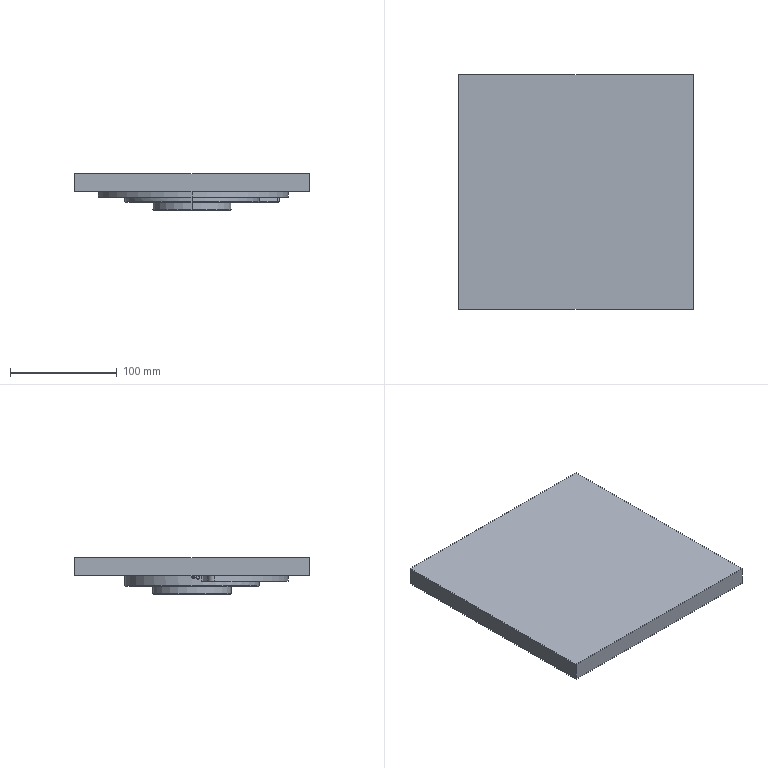NC program | NX | posted with a generic post | part box 220 x 220 x 34.5 mm
Whole program:
N10 G17 G21 G94 G90
(ADAPTIVE_MILLING_COPY , TOOL : D10)
N12 T03 M6
N14 G54
N16 G17 G0 G90 X2.716 Y17.888 S8000 M3
N18 G43 Z30. H3
N20 Z3.
N22 G94 G3 X2.716 Y17.888 Z2.506 I4.346 J1.167 F1000.
N24 X2.716 Y17.888 Z2.013 I4.346 J1.167
N26 X2.716 Y17.888 Z1.519 I4.346 J1.167
N28 X2.716 Y17.888 Z1.026 I4.346 J1.167
N30 X2.716 Y17.888 Z0.532 I4.346 J1.167
N32 X2.716 Y17.888 Z0.039 I4.346 J1.167
N34 X2.716 Y17.888 Z-0.455 I4.346 J1.167
N36 X2.716 Y17.888 Z-0.948 I4.346 J1.167
N38 X2.716 Y17.888 Z-1.442 I4.346 J1.167
N40 X2.716 Y17.888 Z-1.935 I4.346 J1.167
N42 X2.716 Y17.888 Z-2.429 I4.346 J1.167
N44 X2.716 Y17.888 Z-2.922 I4.346 J1.167
N46 X2.716 Y17.888 Z-3.416 I4.346 J1.167
N48 X2.716 Y17.888 Z-3.909 I4.346 J1.167
N50 X2.716 Y17.888 Z-4.403 I4.346 J1.167
N52 X2.716 Y17.888 Z-4.896 I4.346 J1.167
N54 X2.716 Y17.888 Z-5.39 I4.346 J1.167
N56 X2.716 Y17.888 Z-5.884 I4.346 J1.167
N58 X2.716 Y17.888 Z-6.377 I4.346 J1.167
N60 X2.562 Y19.055 Z-6.85 R-4.5
N62 X3.383 Y21.661 R-4.501 F3500.
N64 X8.053 Y14.188 R4.667
N66 X3.478 Y22.528 R-4.976
N68 X8.711 Y13.847 R5.194
N70 X3.384 Y23.139 R-5.476
N72 X9.145 Y13.448 R5.718
N74 X3.268 Y23.733 R-5.999
N76 X9.662 Y13.077 R6.259
N78 X3.411 Y24.511 R-6.54
N80 X10.277 Y12.751 R6.816
N82 X3.54 Y25.251 R-7.101
N84 X10.308 Y12.118 R7.391
N86 X3.277 Y25.774 R-7.685
N88 X9.662 Y11.224 R7.976
N90 X3.634 Y26.625 R-8.28
N92 X9.857 Y10.649 R8.582
N94 X3.931 Y27.41 R-8.89
N96 X9.362 Y9.854 R9.201
N98 X4.542 Y28.271 R-9.52
N100 X8.982 Y9.114 R9.839
N102 X5.936 Y29.188 R10.16
N104 X8.763 Y8.414 R-10.486
N106 X6.773 Y29.902 R10.813
N108 X6.843 Y7.627 R11.141
N110 X9.329 Y30.345 R11.47
N112 X4.111 Y7.333 R11.803
N114 X13.435 Y29.453 R12.135
N116 X-2.975 Y11.336 R12.452
N118 X19.934 Y19.603 R12.744
N120 X-3.247 Y27.048 R12.999
N122 X13.33 Y7.035 R13.282
N124 X3.629 Y32.267 R13.605
N126 X6.415 Y4.841 R13.939
N128 X10.361 Y33.004 R14.279
N130 X0.145 Y5.873 R14.618
N132 X20.504 Y25.811 R14.941
N134 X-7.945 Y22.137 R15.228
N136 X18.812 Y8.559 R15.508
N138 X0.809 Y33.635 R15.819
N140 X8.349 Y2.654 R16.156
N142 X8.223 Y35.578 R16.507
N144 X-0.93 Y3.92 R16.852
N146 X23.417 Y24.631 R17.169
N148 X-9.691 Y24.251 R17.446
N150 X19.666 Y6.189 R17.75
N152 X1.187 Y36.206 R18.081
N154 X6.266 Y0.364 R18.419
N156 X15.685 Y35.789 R18.757
N158 X-9.987 Y10.076 R19.08
N160 X26.272 Y15.384 R19.369
N162 X-1.406 Y36.84 R19.661
N164 X8.189 Y-1.19 R19.988
N166 X14.801 Y37.916 R20.325
N168 X-11.477 Y9.57 R20.641
N170 X27.88 Y15.462 R20.932
N172 X-5.392 Y36.339 R21.244
N174 X11.239 Y-2.415 R21.589
N176 X10.804 Y40.72 R21.927
N178 X-12.156 Y7.506 R22.236
N180 X29.663 Y16.717 R22.529
N182 X-12.155 Y31.619 R22.858
N184 X22.624 Y1.436 R23.224
N186 X0.916 Y41.898 R23.596
N188 X1.166 Y-4.412 R23.935
N190 X30.963 Y23.684 R24.215
N192 X-17.329 Y22.681 R24.515
N194 X29.606 Y7.931 R24.881
N196 X-7.054 Y40.094 R25.257
N198 X9.779 Y-6.692 R25.619
N200 X19.138 Y42.091 R25.939
N202 X-19.073 Y15.618 R26.215
N204 X32.436 Y10.504 R26.54
N206 X-9.113 Y40.665 R26.905
N208 X9.872 Y-8.332 R27.27
N210 X31.353 Y32.222 R27.545
N212 X-20.818 Y16.477 R27.828
N214 X34.139 Y10.383 R28.192
N216 X-13.922 Y38.615 R28.575
N218 X20.169 Y-7.081 R28.964
N220 X11.216 Y48.139 R29.325
N222 X-20.081 Y6.899 R29.589
N224 X37.112 Y17.241 R29.893
N226 X-20.334 Y32.265 R30.27
N228 X35.542 Y6.975 R-30.677
N230 X-10.353 Y44.912 R31.075
N232 X4.684 Y-12.514 R31.429
N234 X38.806 Y20.982 R31.66
N236 X-25.116 Y19.166 R31.992
N238 X38.939 Y12.068 R32.396
N240 X-19.377 Y38.683 R32.793
N242 X26.997 Y-7.815 R33.193
N244 X13.155 Y52.106 R33.559
N246 X-21.757 Y1.048 R33.807
N248 X41.256 Y15.873 R34.126
N250 X-27.369 Y23.479 R34.529
N252 X41.484 Y11.745 R34.949
N254 X-25.661 Y32.893 R35.364
N256 X40.899 Y6.65 R-35.786
N258 X-17.952 Y45.4 R36.198
N260 X8.094 Y-17.705 R36.567
N262 X38.936 Y37.722 R36.804
N264 X-30.067 Y15.176 R37.141
N266 X44.247 Y12.396 R37.546
N268 X13.492 Y56.405 R37.965
N270 X-30.525 Y25.606 R37.965
N272 X44.43 Y9.24 R38.393
N274 X-30.086 Y30.941 R38.821
N276 X44.886 Y7.691 R-39.249
N278 X-28.896 Y36.233 R39.678
N280 X25.894 Y-16.587 R40.091
N282 X22.285 Y56.567 R40.413
N284 X-28.702 Y-0.723 R40.677
N286 X47.754 Y25.827 R41.046
N288 X-34.57 Y20.407 R41.457
N290 X49.119 Y16.929 R41.882
N292 X-34.672 Y27.107 R42.31
N294 X48.583 Y7.952 R42.74
N296 X-32.704 Y36.316 R43.17
N298 X43.357 Y-5.524 R43.591
N300 X-14.118 Y57.762 R43.992
N302 X-10.658 Y-21.75 R44.316
N304 X49.466 Y33.391 R44.581
N306 X-38.078 Y20.459 R44.966
N308 X52.165 Y12.201 R45.389
N310 X-36.223 Y34.618 R45.814
N312 X44.975 Y-7.814 R46.231
N314 X-12.154 Y61.68 R46.627
N316 X-10.656 Y-24.618 R46.947
N318 X52.276 Y33.318 R47.227
N320 X-40.455 Y24.277 R47.612
N322 X54.035 Y7.978 R48.029
N324 X-35.913 Y41.814 R48.452
N326 X7.42 Y-29.926 R48.83
N328 X51.259 Y40.653 R49.041
N330 X-42.314 Y23.549 R49.391
N332 X56.226 Y9.748 R49.806
N334 X-39.088 Y39.358 R50.234
N336 X16.256 Y-30.894 R50.621
N338 X49.884 Y46.721 R50.846
N340 X-44.302 Y19.961 R51.179
N342 X58.321 Y11.441 R51.594
N344 X-41.303 Y38.717 R52.021
N346 X23.088 Y-31.032 R52.413
N348 X52.024 Y46.669 R52.636
N350 X-45.98 Y22.469 R52.961
N352 X54.68 Y-5.516 R53.364
N354 X-35.988 Y51.575 R53.772
N356 X16.02 Y-34.544 R54.152
N358 X56.534 Y42.013 R54.389
N360 X-47.429 Y25.976 R54.737
N362 X41.2 Y-24.486 R55.137
N364 X18.984 Y73.33 R55.465
N366 X-35.269 Y-17.545 R55.766
N368 X61.342 Y34.065 R56.129
N370 X-46.879 Y36.509 R56.511
N372 X29.501 Y-33.423 R56.893
N374 X55.176 Y50.08 R57.13
N376 X-50.244 Y25.13 R57.44
N378 X42.107 Y-27.178 R57.83
N380 X34.431 Y70.449 R58.131
N382 X-46.471 Y-4.811 R58.421
N384 X65.365 Y28.111 R58.801
N386 X-46.387 Y44.91 R59.193
N388 X32.199 Y-35.172 R59.575
N390 X57.762 Y51.058 R59.83
N392 X-53.222 Y21.694 R60.152
N394 X47.578 Y-26.178 R60.54
N396 X10.366 Y79.968 R60.874
N398 X-32.528 Y-27.865 R61.198
N400 X64.036 Y42.837 R61.557
N402 X-52.867 Y35.384 R61.929
N404 X45.069 Y-30.577 R62.315
N406 X44.879 Y69.094 R62.617
N408 X-53.301 Y0.64 R62.918
N410 X70.426 Y23.429 R63.308
N412 X-48.907 Y49.863 R63.706
N414 X34.131 Y-39.257 R64.089
N416 X60.612 Y54.983 R64.36
N418 X33.989 Y77.744 R63.941
N420 G1 X28.698 Y79.849
N422 X28.662 Y79.862
N424 G3 X20.997 Y82.139 R87.113
N426 X-54.045 Y-2.961 R64.765
N428 X48.665 Y-31.222 R65.099
N430 G2 X50.178 Y-29.197 R28.042
N432 X52.808 Y-27.177 R60.231
N434 G3 X60.417 Y-18.593 R46.468
N436 X49.891 Y68.594 R65.492
N438 G1 X48.977 Y69.287
N440 X48.946 Y69.309
N442 X44.187 Y72.436
N444 X44.154 Y72.455
N446 X39.195 Y75.254
N448 X39.161 Y75.272
N450 X36.229 Y76.674
N452 X24.021 Y81.354
N454 X23.204 Y81.615
N456 X17.64 Y82.995
N458 X11.996 Y83.997
N460 X7.521 Y84.475
N462 G3 X0.655 Y84.334 R43.981
N464 X-32.092 Y71.796 R65.284
N466 X-58.559 Y13.61 R65.788
N468 G1 X-58.529 Y13.481
N470 X-58.484 Y13.356
N472 X-58.099 Y12.813
N474 X-57.485 Y11.369
N476 X-57.205 Y9.883
N478 G3 X-57.255 Y6.281 R33.698
N480 X-55.034 Y-2.933 R40.231
N482 X46.954 Y-33.747 R66.001
N484 G1 X48.707 Y-31.16
N486 G3 X48.568 Y-30.401 R0.553
N488 G1 X48.189 Y-30.236 Z-6.829
N490 X47.8 Y-30.098 Z-6.809
N492 X46.7 Y-29.691 Z-6.75
N494 X-54.773 Y7.834
N496 X-56.597 Y8.505 Z-6.847
N498 X-56.652 Y8.516 Z-6.85
N500 G3 X-57.28 Y8.029 R0.552
N502 X-57.562 Y4.17 R25.827
N504 X-55.886 Y-3.248 R30.359
N506 X14.094 Y-47.609 R66.775
N508 X44.952 Y-36.336 R66.922
N510 X47.023 Y-33.645 R32.697
N512 X46.884 Y-32.886 R0.553
N514 G1 X46.507 Y-32.72 Z-6.829
N516 X46.119 Y-32.581 Z-6.809
N518 X45.018 Y-32.17 Z-6.75
N520 X-55.047 Y5.216
N522 X-56.868 Y5.894 Z-6.847
N524 X-56.923 Y5.905 Z-6.85
N526 G3 X-57.553 Y5.419 R0.552
N528 X-56.844 Y-3.055 R18.105
N530 X-47.8 Y-20.796 R61.927
N532 X42.848 Y-38.819 R67.936
N534 X44.964 Y-36.321 R29.568
N536 X44.849 Y-35.524 R0.552
N538 G1 X44.426 Y-35.342 Z-6.827
N540 X43.993 Y-35.186 Z-6.804
N542 X42.983 Y-34.808 Z-6.75
N544 X-55.263 Y1.938
N546 X-57.083 Y2.615 Z-6.847
N548 X-57.14 Y2.627 Z-6.85
N550 G3 X-57.77 Y2.096 R0.552
N552 X-57.77 Y-1.826 R30.463
N554 X-55.602 Y-8.983 R28.364
N556 X-16.913 Y-45.467 R68.138
N558 X40.552 Y-41.236 R68.868
N560 G1 X42.876 Y-38.789
N562 G3 X42.784 Y-37.954 R0.552
N564 G1 X42.272 Y-37.738 Z-6.822
N566 X41.75 Y-37.547 Z-6.794
N568 X40.92 Y-37.233 Z-6.75
N570 X-55.33 Y-0.82
N572 X-57.149 Y-0.135 Z-6.847
N574 X-57.204 Y-0.123 Z-6.85
N576 G3 X-57.84 Y-0.653 R0.552
N578 G1 X-57.844 Y-0.817
N580 X-57.843 Y-0.847
N582 X-57.817 Y-1.329
N584 G3 X-57.502 Y-5.564 R38.929
N586 X-54.651 Y-13.147 R30.654
N588 X-0.182 Y-50.379 R69.435
N590 X37.85 Y-43.693 R69.779
N592 X40.625 Y-41.159 R57.486
N594 X40.529 Y-40.321 R0.552
N596 G1 X40.016 Y-40.108 Z-6.822
N598 X39.493 Y-39.919 Z-6.794
N600 X38.661 Y-39.608 Z-6.75
N602 X-55.129 Y-4.569
N604 X-56.064 Y-4.215 Z-6.8
N606 X-57.005 Y-3.878 Z-6.85
N608 G3 X-57.649 Y-4.449 R0.552
N610 X-56.899 Y-9.724 R29.781
N612 X-53.157 Y-17.747 R36.163
N614 X34.904 Y-46.072 R70.603
N616 X37.854 Y-43.69 R29.715
N618 X37.766 Y-42.805 R0.551
N620 G1 X35.894 Y-42.101 Z-6.75
N622 X-54.654 Y-8.467
N624 X-56.53 Y-7.775 Z-6.85
N626 G3 X-57.198 Y-8.383 R0.551
N628 X-55.894 Y-14.167 R25.106
N630 X-50.72 Y-23.133 R44.051
N632 X31.686 Y-48.351 R71.626
N634 X34.937 Y-46.048 R32.018
N636 X34.839 Y-45.111 R0.551
N638 G1 X32.962 Y-44.42 Z-6.75
N640 X-53.857 Y-12.553
N642 X-55.735 Y-11.865 Z-6.85
N644 G3 X-56.437 Y-12.505 R0.551
N646 X-54.12 Y-19.416 R23.57
N648 X-45.519 Y-30.887 R56.893
N650 X28.12 Y-50.522 R72.643
N652 X31.778 Y-48.293 R44.276
N654 X31.649 Y-47.303 R0.551
N656 G1 X29.77 Y-46.619 Z-6.75
N658 X-52.751 Y-16.584
N660 X-54.631 Y-15.9 Z-6.85
N662 G3 X-55.382 Y-16.561 R0.552
N664 X-52.775 Y-23.11 R26.971
N666 X-44.509 Y-33.264 R54.486
N668 X24.096 Y-52.568 R73.579
N670 X28.148 Y-50.507 R58.714
N672 X28.079 Y-49.502 R0.551
N674 G1 X27.96 Y-49.459
N676 X26.078 Y-48.782 Z-6.75
N678 X-51.16 Y-21.
N680 X-53.042 Y-20.323 Z-6.85
N682 G3 X-53.84 Y-20.561 R0.584
N684 X-53.857 Y-20.997 R0.574
N686 X-50.497 Y-27.756 R29.648
N688 X-40.677 Y-38.034 R58.333
N690 X19.4 Y-54.467 R74.543
N692 G1 X20.294 Y-54.173
N694 X20.337 Y-54.156
N696 X24.137 Y-52.55
N698 G3 X24.107 Y-51.526 R0.551
N700 G1 X23.854 Y-51.436
N702 X21.969 Y-50.766 Z-6.75
N704 X-49.082 Y-25.512
N706 X-50.966 Y-24.843 Z-6.85
N708 X-51.199 Y-24.761
N710 X-51.445 Y-24.737
N712 G3 X-51.869 Y-25.52 R0.551
N714 X-48.329 Y-31.628 R40.408
N716 X-40.346 Y-39.52 R50.034
N718 X13.863 Y-56.115 R75.438
N720 G1 X15.777 Y-55.656
N722 X15.822 Y-55.643
N724 X19.503 Y-54.433
N726 G3 X19.513 Y-53.391 R0.55
N728 G1 X19.067 Y-53.235
N730 X17.18 Y-52.573 Z-6.75
N732 X-46.272 Y-30.31
N734 X-48.159 Y-29.647 Z-6.85
N736 X-48.681 Y-29.472
N738 G3 X-49.252 Y-30.291 R0.551
N740 G1 X-48.798 Y-31.068
N742 X-48.775 Y-31.106
N744 X-46.194 Y-34.823
N746 X-46.167 Y-34.858
N748 G3 X-39.576 Y-41.312 R36.113
N750 X7.33 Y-57.354 R76.215
N752 G1 X11.154 Y-56.764
N754 X11.2 Y-56.755
N756 X13.874 Y-56.113
N758 G3 X13.92 Y-55.057 R0.55
N760 G1 X13.176 Y-54.807
N762 X11.28 Y-54.171 Z-6.75
N764 X-41.641 Y-36.428
N766 X-43.538 Y-35.792 Z-6.85
N768 X-44.386 Y-35.515
N770 G3 X-44.901 Y-36.406 R0.551
N772 G1 X-43.302 Y-38.36
N774 X-43.272 Y-38.393
N776 X-40.139 Y-41.658
N778 X-40.107 Y-41.689
N780 G3 X-31.074 Y-48.139 R47.059
N782 X-1.616 Y-57.787 R77.307
N784 G1 X1.714 Y-57.824
N786 X1.76 Y-57.822
N788 X6.456 Y-57.488
N790 X6.502 Y-57.483
N792 X7.367 Y-57.349
N794 G3 X7.446 Y-56.28 R0.55
N796 G1 X5.785 Y-55.764
N798 X3.875 Y-55.171 Z-6.75
N800 X-34.475 Y-43.257
N802 X-36.385 Y-42.664 Z-6.85
N804 X-38.076 Y-42.146
N806 G3 X-38.519 Y-43.101 R0.55
N808 G1 X-36.726 Y-44.696
N810 X-36.691 Y-44.724
N812 X-33.083 Y-47.455
N814 X-33.047 Y-47.481
N816 X-29.235 Y-49.919
N818 X-29.196 Y-49.941
N820 X-25.203 Y-52.07
N822 X-25.163 Y-52.09
N824 X-21.015 Y-53.897
N826 X-20.974 Y-53.913
N828 X-16.695 Y-55.388
N830 X-16.653 Y-55.4
N832 X-12.272 Y-56.533
N834 X-12.228 Y-56.542
N836 X-7.772 Y-57.325
N838 X-7.727 Y-57.331
N840 X-3.039 Y-57.769
N842 X-2.993 Y-57.772
N844 X-1.493 Y-57.788
N846 X-1.352 Y-57.768
N848 X-1.218 Y-57.718
N850 X1.509 Y-56.188
N852 X3.254 Y-55.21 Z-6.75
N854 X45.409 Y-31.565
N856 X47.154 Y-30.587 Z-6.85
N858 X51.374 Y-28.22
N860 X51.396 Y-28.208
N862 G3 X54.205 Y-26.698 R21.883
N864 X59.618 Y-21.184 R28.83
N866 X72.222 Y31.316 R65.863
N868 X57.005 Y62.807 R66.863
N870 X49.829 Y68.64 R80.223
N872 X48.949 Y68.134 R0.552
N874 G1 X49.016 Y66.135 Z-6.75
N876 X52.054 Y-25.113
N878 X52.122 Y-27.053 Z-6.847
N880 X52.133 Y-27.111 Z-6.85
N882 G3 X52.8 Y-27.508 R0.553
N884 X56.743 Y-25.459 R8.272
N886 X62.894 Y-18.253 R36.756
N888 X61.924 Y58.007 R67.156
N890 G1 X61.898 Y58.034
N892 X57.866 Y62.056
N894 X57.838 Y62.082
N896 X56.99 Y62.82
N898 G3 X56.077 Y62.375 R0.553
N900 G1 X56.008 Y60.376 Z-6.75
N902 X53.031 Y-24.859
N904 X52.966 Y-26.8 Z-6.847
N906 X52.973 Y-26.858 Z-6.85
N908 G3 X53.649 Y-27.295 R0.552
N910 G1 X54.263 Y-27.141
N912 X54.324 Y-27.132
N914 X54.449 Y-27.129
N916 X54.573 Y-27.115
N918 X54.696 Y-27.093
N920 X54.818 Y-27.066
N922 X54.94 Y-27.037
N924 X55.06 Y-27.003
N926 X55.179 Y-26.965
N928 G3 X59.07 Y-24.303 R11.344
N930 X66.021 Y-15.028 R44.175
N932 X66.244 Y52.98 R68.174
N934 G1 X65.7 Y53.693
N936 X65.676 Y53.722
N938 X62.053 Y57.86
N940 G3 X61.091 Y57.545 R0.551
N942 G1 X61.077 Y57.386
N944 X60.907 Y55.394 Z-6.75
N946 X54.049 Y-24.636
N948 X53.886 Y-26.629 Z-6.85
N950 G3 X54.449 Y-27.129 R0.553
N952 X58.177 Y-25.911 R5.856
N954 X63.347 Y-20.693 R24.137
N956 X73.335 Y-0.385 R64.082
N958 X69.673 Y48.381 R69.131
N960 X66.197 Y53.041 R83.217
N962 X65.215 Y52.779 R0.551
N964 G1 X65.189 Y52.587
N966 X64.928 Y50.604 Z-6.75
N968 X55.012 Y-24.598
N970 X54.759 Y-26.581 Z-6.85
N972 G3 X55.323 Y-27.106 R0.553
N974 X59.038 Y-26.039 R5.782
N976 X64.205 Y-21.002 R21.991
N978 X72.844 Y-4.862 R61.211
N980 X72.539 Y43.992 R70.021
N982 X69.628 Y48.45 R396.035
N984 X68.627 Y48.242 R0.551
N986 G1 X68.586 Y48.01
N988 X68.239 Y46.041 Z-6.75
N990 X55.786 Y-24.574
N992 X55.445 Y-26.544 Z-6.85
N994 G3 X55.889 Y-27.097 R0.554
N996 X59.032 Y-26.658 R4.332
N998 X63.769 Y-22.834 R15.987
N1000 X70.769 Y-12.074 R48.624
N1002 X75.005 Y39.652 R70.807
N1004 G1 X72.535 Y44.
N1006 G3 X71.52 Y43.846 R0.551
N1008 G1 X71.459 Y43.568
N1010 X71.03 Y41.614 Z-6.75
N1012 X56.489 Y-24.651
N1014 X56.063 Y-26.605 Z-6.85
N1016 G3 X56.502 Y-27.217 R0.553
N1018 X60.01 Y-26.768 R4.73
N1020 X64.924 Y-22.769 R16.622
N1022 X71.749 Y-12.191 R47.773
N1024 X77.137 Y35.275 R71.619
N1026 G1 X75.147 Y39.399
N1028 X75.13 Y39.433
N1030 X74.944 Y39.759
N1032 G3 X73.934 Y39.625 R0.551
N1034 G1 X73.856 Y39.323
N1036 X73.356 Y37.387 Z-6.75
N1038 X57.296 Y-24.808
N1040 X56.799 Y-26.745 Z-6.85
N1042 G3 X57.238 Y-27.361 R0.553
N1044 X60.232 Y-27.227 R4.02
N1046 X65.173 Y-23.689 R14.26
N1048 X71.427 Y-14.831 R41.208
N1050 X78.939 Y30.994 R72.072
N1052 X77.116 Y35.318 R55.462
N1054 X76.095 Y35.239 R0.551
N1056 G1 X76.011 Y34.964
N1058 X75.43 Y33.051 Z-6.75
N1060 X57.813 Y-24.907
N1062 X57.232 Y-26.821 Z-6.85
N1064 G3 X57.545 Y-27.456 R0.554
N1066 X60.577 Y-27.622 R3.764
N1068 X65.396 Y-24.575 R12.82
N1070 X71.759 Y-16.114 R36.775
N1072 X80.785 Y22.207 R71.989
N1074 X80.445 Y26.838 R122.758
N1076 X78.938 Y30.994 R40.273
N1078 X77.908 Y30.969 R0.551
N1080 G1 X77.801 Y30.66
N1082 X77.147 Y28.77 Z-6.75
N1084 X58.476 Y-25.127
N1086 X57.821 Y-27.017 Z-6.85
N1088 G3 X58.118 Y-27.708 R0.553
N1090 X61.391 Y-27.882 R4.062
N1092 X66.411 Y-24.688 R13.321
N1094 X72.82 Y-16.105 R36.835
N1096 X81.79 Y19.38 R72.433
N1098 G1 X81.787 Y19.88
N1100 X81.781 Y20.38
N1102 X81.772 Y20.879
N1104 X81.76 Y21.379
N1106 X81.743 Y21.879
N1108 X81.728 Y22.254
N1110 X81.701 Y22.814
N1112 G3 X80.413 Y26.937 R62.817
N1114 X79.377 Y26.965 R0.551
N1116 G1 X79.234 Y26.594
N1118 X78.512 Y24.729 Z-6.75
N1120 X59.115 Y-25.404
N1122 X58.393 Y-27.269 Z-6.85
N1124 G3 X58.69 Y-27.959 R0.553
N1126 X61.76 Y-28.286 R3.815
N1128 X66.709 Y-25.463 R12.335
N1130 X72.944 Y-17.695 R32.876
N1132 X81.544 Y5.77 R70.004
N1134 X82.728 Y18.763 R77.216
N1136 G1 X81.684 Y22.882
N1138 G3 X80.646 Y22.966 R0.55
N1140 G1 X80.46 Y22.536
N1142 X79.666 Y20.7 Z-6.75
N1144 X59.633 Y-25.628
N1146 X58.84 Y-27.464 Z-6.85
N1148 G3 X59.07 Y-28.157 R0.554
N1150 X62.178 Y-28.683 R3.814
N1152 X67.219 Y-26.036 R11.879
N1154 X73.715 Y-18.165 R31.792
N1156 X82.041 Y3.425 R68.847
N1158 X83.539 Y14.599 R78.021
N1160 X82.714 Y18.818 R64.758
N1162 X81.685 Y18.92 R0.551
N1164 G1 X81.484 Y18.499
N1166 X80.622 Y16.694 Z-6.75
N1168 X60.256 Y-25.942
N1170 X59.394 Y-27.747 Z-6.85
N1172 G3 X59.611 Y-28.47 R0.554
N1174 X62.958 Y-29.019 R4.048
N1176 X68.102 Y-26.298 R12.318
N1178 X74.543 Y-18.542 R31.69
N1180 X82.655 Y1.807 R68.753
N1182 X84.143 Y10.6 R79.303
N1184 X83.52 Y14.703 R38.965
N1186 X82.491 Y14.859 R0.551
N1188 G1 X82.281 Y14.457
N1190 X81.356 Y12.684 Z-6.75
N1192 X60.968 Y-26.352
N1194 X60.042 Y-28.125 Z-6.85
N1196 G3 X60.261 Y-28.845 R0.553
N1198 X63.613 Y-29.392 R4.146
N1200 X68.983 Y-26.573 R12.602
N1202 X75.691 Y-18.395 R32.519
N1204 X83.555 Y1.523 R68.964
N1206 X84.574 Y6.833 R76.032
N1208 G1 X84.133 Y10.683
N1210 G3 X83.109 Y10.893 R0.55
N1212 G1 X82.846 Y10.433
N1214 X81.852 Y8.698 Z-6.75
N1216 X61.576 Y-26.703
N1218 X60.583 Y-28.439 Z-6.85
N1220 G3 X60.802 Y-29.157 R0.553
N1222 X64.386 Y-29.752 R4.321
N1224 X69.955 Y-26.779 R13.154
N1226 X76.766 Y-18.363 R33.391
N1228 X84.77 Y2.666 R70.068
N1230 G1 X84.577 Y6.786
N1232 G3 X83.578 Y7.047 R0.541
N1234 G1 X83.169 Y6.39
N1236 X82.112 Y4.693 Z-6.75
N1238 X62.297 Y-27.118
N1240 X61.241 Y-28.817 Z-6.85
N1242 G3 X61.451 Y-29.532 R0.543
N1244 X65.036 Y-30.145 R4.367
N1246 X70.538 Y-27.308 R13.1
N1248 X77.387 Y-19.086 R32.713
N1250 X84.793 Y-1.298 R68.093
N1252 X84.766 Y2.768 R39.621
N1254 X83.761 Y3.051 R0.55
N1256 G1 X83.288 Y2.354
N1258 X82.164 Y0.699 Z-6.75
N1260 X63.004 Y-27.527
N1262 X61.884 Y-29.184 Z-6.85
N1264 G3 X62.101 Y-29.907 R0.553
N1266 X65.683 Y-30.546 R4.421
N1268 X71.406 Y-27.603 R13.294
N1270 X78.131 Y-19.6 R32.453
N1272 X84.686 Y-5.036 R65.018
N1274 X84.796 Y-1.174 R181.103
N1276 X83.804 Y-0.835 R0.55
N1278 G1 X83.404 Y-1.375
N1280 X82.213 Y-2.982 Z-6.75
N1282 X63.722 Y-27.941
N1284 X62.538 Y-29.552 Z-6.85
N1286 G3 X62.751 Y-30.282 R0.553
N1288 X66.453 Y-30.926 R4.533
N1290 X72.085 Y-28.067 R13.517
N1292 X78.938 Y-20.011 R32.265
N1294 X84.35 Y-8.866 R61.683
N1296 G1 X84.689 Y-5.005
N1298 G3 X83.714 Y-4.611 R0.55
N1300 G1 X83.301 Y-5.119
N1302 X82.041 Y-6.673 Z-6.75
N1304 X64.446 Y-28.358
N1306 X63.193 Y-29.917 Z-6.85
N1308 G3 X63.4 Y-30.657 R0.553
N1310 X67.099 Y-31.336 R4.566
N1312 X72.758 Y-28.533 R13.506
N1314 X79.678 Y-20.534 R32.182
N1316 X83.868 Y-12.564 R58.873
N1318 X84.352 Y-8.851 R38.627
N1320 X83.392 Y-8.437 R0.55
N1322 G1 X83.017 Y-8.86
N1324 X81.689 Y-10.355 Z-6.75
N1326 X65.277 Y-28.839
N1328 X63.987 Y-30.296 Z-6.847
N1330 X63.958 Y-30.342 Z-6.85
N1332 G3 X64.158 Y-31.095 R0.553
N1334 X67.742 Y-31.751 R4.539
N1336 X73.526 Y-28.925 R13.481
N1338 X80.614 Y-20.745 R32.444
N1340 X83.359 Y-15.83 R58.223
N1342 G1 X83.878 Y-12.496
N1344 G3 X82.943 Y-12.026 R0.55
N1346 G1 X82.545 Y-12.43
N1348 X81.144 Y-13.857 Z-6.75
N1350 X66.011 Y-29.263
N1352 X64.652 Y-30.651 Z-6.847
N1354 X64.619 Y-30.698 Z-6.85
N1356 G3 X64.807 Y-31.47 R0.552
N1358 X68.507 Y-32.149 R4.599
N1360 X74.491 Y-29.171 R13.926
N1362 X81.612 Y-20.853 R33.251
N1364 G1 X81.81 Y-20.535
N1366 X82.006 Y-20.215
N1368 X82.199 Y-19.894
N1370 X82.453 Y-19.463
N1372 X82.578 Y-19.246
N1374 X82.604 Y-19.191
N1376 X83.349 Y-15.884
N1378 X83.356 Y-15.847
N1380 X83.376 Y-15.723
N1382 G3 X82.458 Y-15.236 R0.551
N1384 G1 X82.003 Y-15.658
N1386 X80.538 Y-17.02 Z-6.75
N1388 X66.846 Y-29.746
N1390 X65.425 Y-31.07 Z-6.847
N1392 X65.389 Y-31.116 Z-6.85
N1394 G3 X65.565 Y-31.907 R0.552
N1396 X69.151 Y-32.568 R4.589
N1398 X75.062 Y-29.724 R13.636
N1400 X81.927 Y-22.009 R31.534
N1402 X82.628 Y-19.085 R62.911
N1404 X81.742 Y-18.539 R0.551
N1406 G1 X81.388 Y-18.831
N1408 X79.844 Y-20.102 Z-6.75
N1410 X67.599 Y-30.181
N1412 X66.099 Y-31.419 Z-6.847
N1414 X66.062 Y-31.46 Z-6.85
N1416 G3 X66.215 Y-32.282 R0.552
N1418 X69.917 Y-32.973 R4.683
N1420 X75.929 Y-30.054 R13.949
N1422 X81.146 Y-24.638 R28.596
N1424 G1 X81.929 Y-22.002
N1426 G3 X81.079 Y-21.4 R0.55
N1428 G1 X80.697 Y-21.677
N1430 X79.077 Y-22.851 Z-6.75
N1432 X68.357 Y-30.619
N1434 X66.743 Y-31.799 Z-6.85
N1436 G3 X66.864 Y-32.657 R0.552
N1438 X70.681 Y-33.38 R4.777
N1440 X76.698 Y-30.465 R14.136
N1442 X80.507 Y-26.788 R24.792
N1444 G1 X81.148 Y-24.631
N1446 G3 X80.324 Y-24.011 R0.551
N1448 G1 X80.043 Y-24.191
N1450 X78.358 Y-25.27 Z-6.75
N1452 X69.22 Y-31.118
N1454 X67.539 Y-32.201 Z-6.85
N1456 G3 X67.622 Y-33.095 R0.551
N1458 X71.321 Y-33.813 R4.718
N1460 X76.961 Y-31.251 R13.704
N1462 X79.754 Y-28.832 R18.88
N1464 G1 X80.474 Y-26.896
N1466 X80.486 Y-26.861
N1468 X80.521 Y-26.741
N1470 G3 X79.721 Y-26.106 R0.551
N1472 G1 X79.417 Y-26.28
N1474 X77.68 Y-27.272 Z-6.75
N1476 X70.08 Y-31.609
N1478 X68.344 Y-32.602 Z-6.85
N1480 G3 X68.38 Y-33.532 R0.551
N1482 X72.084 Y-34.225 R4.746
N1484 X77.829 Y-31.594 R13.989
N1486 X79.14 Y-30.485 R6.86
N1488 G1 X79.793 Y-28.727
N1490 G3 X79.035 Y-28.042 R0.551
N1492 G1 X78.823 Y-28.146
N1494 X77.028 Y-29.027 Z-6.75
N1496 X70.855 Y-32.057
N1498 X69.06 Y-32.938 Z-6.85
N1500 G3 X69.029 Y-33.907 R0.551
N1502 X72.847 Y-34.642 R4.847
N1504 X78.558 Y-31.963 R12.994
N1506 X79.153 Y-30.449 R20.278
N1508 X78.424 Y-29.75 R0.551
N1510 G1 X78.292 Y-29.806
N1512 X76.449 Y-30.582 Z-6.75
N1514 X71.735 Y-32.567
N1516 X69.892 Y-33.343 Z-6.85
N1518 G3 X69.787 Y-34.345 R0.552
N1520 X73.607 Y-35.061 R4.837
N1522 X77.968 Y-33.274 R11.136
N1524 X78.633 Y-31.847 R5.407
N1526 X77.93 Y-31.138 R0.551
N1528 G1 X70.551 Y-33.826
N1530 G3 X70.545 Y-34.782 R0.551
N1532 X74.122 Y-35.519 R4.708
N1534 X77.506 Y-34.31 R8.108
N1536 X78.122 Y-33.047 R6.467
N1538 X77.454 Y-32.297 R0.551
N1540 G1 X71.327 Y-34.254
N1542 G3 X71.303 Y-35.22 R0.551
N1544 X75.131 Y-35.898 R4.858
N1546 X77.112 Y-35.176 R5.182
N1548 X77.633 Y-34.134 R4.548
N1550 X76.999 Y-33.375 R0.551
N1552 G1 X72.013 Y-34.612
N1554 G3 X71.952 Y-35.595 R0.551
N1556 X76.797 Y-35.874 R4.503
N1558 X77.268 Y-34.944 R3.882
N1560 X76.648 Y-34.182 R0.551
N1562 G1 X72.782 Y-35.045
N1564 G3 X72.71 Y-36.032 R0.551
N1566 X76.377 Y-36.541 R3.866
N1568 G1 X76.662 Y-36.291
N1570 X76.918 Y-35.721
N1572 G3 X76.316 Y-34.954 R0.551
N1574 G1 X73.556 Y-35.476
N1576 G3 X73.468 Y-36.47 R0.551
N1578 X75.94 Y-37.054 R3.135
N1580 X76.673 Y-36.265 R1.04
N1582 X76.072 Y-35.498 R0.551
N1584 G1 X74.206 Y-35.851
N1586 G3 X74.117 Y-36.845 R0.551
N1588 X75.871 Y-37.327 R2.334
N1590 X76.484 Y-36.685 R0.859
N1592 X75.869 Y-35.921 R0.551
N1594 G1 X74.735 Y-36.168
N1596 G3 X74.658 Y-37.157 R0.551
N1598 X75.942 Y-37.482 R1.536
N1600 X76.342 Y-37.001 R0.823
N1602 X75.669 Y-36.252 R0.551
N1604 G1 X75.111 Y-36.444
N1606 G3 X75.091 Y-37.407 R0.551
N1608 X76.147 Y-37.4 R0.754
N1610 G1 X76.211 Y-37.293
N1612 X76.262 Y-37.179
N1614 G3 X75.923 Y-36.336 R0.642
N1616 X75.078 Y-36.679 R0.642
N1618 X75.359 Y-37.562 R0.691
N1620 X75.979 Y-37.544 R0.634
N1622 X76.182 Y-36.8 R0.553
N1624 G1 X75.778 Y-36.082
N1626 X74.798 Y-34.338 Z-6.75
N1628 X9.562 Y81.738
N1630 X8.582 Y83.482 Z-6.85
N1632 X8.142 Y84.251
N1634 G3 X7.77 Y84.456 R0.576
N1636 G1 X6.334 Y84.613
N1638 X6.296 Y84.615
N1640 X0.583 Y84.848
N1642 G3 X-10.154 Y83.348 R40.247
N1644 X-59.57 Y15.083 R66.563
N1646 X-59.013 Y14.088 R1.206
N1648 G1 X-58.427 Y13.278
N1650 G3 X-57.651 Y13.161 R0.553
N1652 G1 X-57.377 Y13.469 Z-6.829
N1654 X-57.125 Y13.795 Z-6.809
N1656 X-56.394 Y14.715 Z-6.75
N1658 X-2.772 Y82.249
N1660 X-1.528 Y83.816 Z-6.85
N1662 G3 X-1.916 Y84.781 R0.558
N1664 X-10.62 Y84.041 R48.968
N1666 X-25.036 Y78.475 R57.326
N1668 X-60.584 Y16.78 R67.519
N1670 X-60.254 Y15.204 R3.73
N1672 G1 X-60.216 Y15.156
N1674 X-60.184 Y15.133
N1676 X-59.341 Y14.388
N1678 G3 X-58.602 Y14.397 R0.554
N1680 G1 X-58. Y15.196 Z-6.8
N1682 X-57.417 Y16.007 Z-6.75
N1684 X-9.528 Y81.758
N1686 X-8.35 Y83.375 Z-6.85
N1688 G3 X-8.292 Y84.149 R0.595
N1690 X-8.771 Y84.35 R0.561
N1692 X-16.519 Y83.099 R48.801
N1694 X-28.734 Y77.436 R53.541
N1696 X-61.551 Y18.288 R68.457
N1698 X-61.075 Y15.725 R6.667
N1700 X-60.184 Y15.133 R2.829
N1702 X-59.486 Y15.186 R0.554
N1704 G1 X-59.107 Y15.717 Z-6.817
N1706 X-58.748 Y16.264 Z-6.785
N1708 X-58.363 Y16.839 Z-6.75
N1710 X-15.477 Y80.856
N1712 X-14.364 Y82.518 Z-6.85
N1714 G3 X-14.18 Y83.003 R0.735
N1716 X-14.817 Y83.505 R0.552
N1718 X-21.855 Y81.875 R49.543
N1720 X-31.969 Y76.458 R48.761
N1722 X-62.485 Y19.723 R69.341
N1724 X-61.944 Y16.289 R8.96
N1726 X-61.554 Y15.898 R0.785
N1728 G1 X-60.898 Y15.535
N1730 G3 X-60.181 Y15.702 R0.554
N1732 G1 X-59.136 Y17.408 Z-6.75
N1734 X-21.1 Y79.581
N1736 X-20.056 Y81.287 Z-6.85
N1738 X-19.938 Y81.486
N1740 X-19.87 Y81.706
N1742 G3 X-20.543 Y82.286 R0.551
N1744 X-26.974 Y80.319 R43.935
N1746 X-36.08 Y74.649 R47.615
N1748 X-63.394 Y21.091 R70.287
N1750 X-62.855 Y16.901 R11.531
N1752 X-62.273 Y16.115 R1.432
N1754 G1 X-61.611 Y15.922
N1756 G3 X-60.996 Y16.149 R0.555
N1758 G1 X-60.014 Y17.891 Z-6.75
N1760 X-26.16 Y78.058
N1762 X-25.179 Y79.801 Z-6.85
N1764 G3 X-24.983 Y80.274 R1.1
N1766 X-25.694 Y80.82 R0.551
N1768 X-32.082 Y78.359 R35.485
N1770 X-41.832 Y70.989 R51.684
N1772 X-64.283 Y22.272 R71.086
N1774 X-63.797 Y17.57 R14.192
N1776 X-63.121 Y16.391 R2.851
N1778 G1 X-63.016 Y16.332
N1780 X-62.176 Y16.087
N1782 G3 X-61.506 Y16.415 R0.559
N1784 G1 X-60.593 Y18.194 Z-6.75
N1786 X-30.762 Y76.346
N1788 X-29.849 Y78.126 Z-6.85
N1790 X-29.736 Y78.342
N1792 X-29.652 Y78.571
N1794 G3 X-30.392 Y79.168 R0.551
N1796 X-36.189 Y76.582 R34.927
N1798 X-44.359 Y69.825 R47.
N1800 X-65.154 Y23.521 R71.888
N1802 X-64.687 Y18.068 R16.41
N1804 X-63.851 Y16.552 R3.669
N1806 X-62.953 Y16.314 R3.201
N1808 X-62.279 Y16.654 R0.557
N1810 G1 X-61.431 Y18.466 Z-6.75
N1812 X-35.268 Y74.361
N1814 X-34.42 Y76.173 Z-6.85
N1816 X-34.298 Y76.424
N1818 X-34.211 Y76.689
N1820 G3 X-34.988 Y77.25 R0.551
N1822 X-39.671 Y74.926 R41.794
N1824 X-46.69 Y68.743 R40.451
N1826 X-66.015 Y24.591 R72.644
N1828 X-65.606 Y18.632 R18.423
N1830 X-64.564 Y16.671 R4.204
N1832 X-63.654 Y16.453 R2.912
N1834 X-63.018 Y16.861 R0.57
N1836 G1 X-62.232 Y18.7 Z-6.75
N1838 X-39.334 Y72.289
N1840 X-38.548 Y74.128 Z-6.85
N1842 X-38.339 Y74.637
N1844 G3 X-39.137 Y75.25 R0.551
N1846 X-43.481 Y72.78 R53.383
N1848 X-49.827 Y66.604 R38.362
N1850 X-66.896 Y25.212 R73.211
N1852 X-66.479 Y19.004 R19.415
N1854 X-65.339 Y16.813 R4.773
N1856 X-64.293 Y16.566 R3.199
N1858 X-63.651 Y16.995 R0.573
N1860 G1 X-62.917 Y18.856 Z-6.75
N1862 X-42.561 Y70.464
N1864 X-41.827 Y72.325 Z-6.85
N1866 X-41.627 Y72.854
N1868 G3 X-42.428 Y73.453 R0.551
N1870 X-47.343 Y70.277 R44.052
N1872 X-53.452 Y63.526 R39.968
N1874 X-67.739 Y26.296 R73.915
N1876 X-67.414 Y19.582 R21.58
N1878 X-66.192 Y17.013 R5.751
N1880 G1 X-66.095 Y16.935
N1882 X-65.985 Y16.876
N1884 X-65.936 Y16.856
N1886 X-65.074 Y16.704
N1888 G3 X-64.439 Y17.121 R0.56
N1890 G1 X-63.77 Y19.006 Z-6.75
N1892 X-46.356 Y68.046
N1894 X-45.687 Y69.931 Z-6.85
N1896 X-45.505 Y70.465
N1898 G3 X-46.342 Y71.025 R0.551
N1900 X-51.42 Y67.223 R28.176
N1902 X-58.073 Y58.336 R49.565
N1904 X-68.59 Y27.21 R74.595
N1906 X-68.312 Y19.995 R23.487
N1908 X-67.021 Y17.184 R6.416
N1910 G1 X-66.929 Y17.099
N1912 X-66.822 Y17.034
N1914 X-66.732 Y16.996
N1916 X-65.871 Y16.844
N1918 G3 X-65.24 Y17.252 R0.555
N1920 G1 X-64.635 Y19.159 Z-6.75
N1922 X-49.952 Y65.418
N1924 X-49.347 Y67.324 Z-6.85
N1926 X-49.156 Y67.95
N1928 G3 X-50.026 Y68.475 R0.551
N1930 X-53.844 Y65.48 R36.5
N1932 X-59.258 Y58.161 R38.368
N1934 X-69.447 Y27.953 R74.844
N1936 X-69.2 Y20.364 R24.544
N1938 X-67.826 Y17.32 R6.699
N1940 G1 X-67.733 Y17.237
N1942 X-67.625 Y17.173
N1944 X-67.545 Y17.139
N1946 X-66.683 Y16.987
N1948 G3 X-66.055 Y17.389 R0.554
N1950 G1 X-65.509 Y19.313 Z-6.75
N1952 X-53.145 Y62.835
N1954 X-52.599 Y64.759 Z-6.85
N1956 X-52.394 Y65.507
N1958 G3 X-53.295 Y65.991 R0.551
N1960 X-56.871 Y62.868 R53.342
N1962 X-61.516 Y56.072 R35.229
N1964 X-70.32 Y28.502 R74.701
N1966 X-70.08 Y20.663 R25.395
N1968 X-68.676 Y17.496 R7.148
N1970 G1 X-68.588 Y17.407
N1972 X-68.485 Y17.337
N1974 X-68.364 Y17.284
N1976 X-67.502 Y17.132
N1978 G3 X-66.876 Y17.529 R0.554
N1980 G1 X-66.382 Y19.467 Z-6.75
N1982 X-55.937 Y60.393
N1984 X-55.443 Y62.331 Z-6.85
N1986 X-55.254 Y63.097
N1988 G3 X-56.157 Y63.568 R0.551
N1990 X-60.231 Y59.546 R33.885
N1992 X-64.725 Y51.768 R42.165
N1994 X-71.262 Y28.276 R72.78
N1996 X-70.839 Y20.449 R23.715
N1998 X-69.425 Y17.561 R6.504
N2000 G1 X-69.323 Y17.489
N2002 X-69.194 Y17.43
N2004 X-68.332 Y17.278
N2006 G3 X-67.707 Y17.671 R0.554
N2008 G1 X-67.275 Y19.624 Z-6.75
N2010 X-58.91 Y57.509
N2012 X-58.479 Y59.462 Z-6.85
N2014 X-58.313 Y60.249
N2016 G3 X-59.245 Y60.675 R0.551
N2018 X-62.961 Y56.657 R28.966
N2020 X-67.369 Y47.982 R44.609
N2022 X-72.17 Y28.38 R70.625
N2024 X-71.68 Y20.558 R23.568
N2026 X-70.233 Y17.687 R6.369
N2028 X-69.161 Y17.424 R2.945
N2030 X-68.537 Y17.816 R0.554
N2032 G1 X-68.167 Y19.781 Z-6.75
N2034 X-61.693 Y54.473
N2036 X-61.326 Y56.439 Z-6.85
N2038 X-61.161 Y57.363
N2040 G3 X-62.119 Y57.744 R0.551
N2042 X-65.15 Y54.253 R46.518
N2044 X-68.825 Y46.75 R35.86
N2046 X-73.071 Y28.547 R68.238
N2048 X-72.539 Y20.728 R23.42
N2050 X-71.098 Y17.852 R6.579
N2052 X-70.009 Y17.574 R2.699
N2054 X-69.385 Y17.966 R0.554
N2056 G1 X-69.065 Y19.94 Z-6.75
N2058 X-63.974 Y51.783
N2060 X-63.658 Y53.758 Z-6.85
N2062 X-63.502 Y54.776
N2064 G3 X-64.461 Y55.143 R0.551
N2066 X-67.874 Y50.701 R39.423
N2068 X-71.245 Y42.511 R40.01
N2070 X-74.034 Y27.559 R60.246
N2072 X-73.208 Y20.27 R20.865
N2074 X-71.941 Y17.996 R5.976
N2076 X-70.857 Y17.723 R2.802
N2078 X-70.231 Y18.117 R0.554
N2080 G1 X-69.981 Y20.101 Z-6.75
N2082 X-66.484 Y48.578
N2084 X-66.24 Y50.563 Z-6.85
N2086 X-66.129 Y51.527
N2088 G3 X-67.111 Y51.844 R0.551
N2090 X-70.519 Y46.792 R26.535
N2092 X-73.789 Y36.444 R49.027
N2094 X-74.894 Y25.031 R43.706
N2096 X-73.558 Y19.224 R14.897
N2098 X-72.646 Y18.056 R2.94
N2100 G1 X-72.577 Y18.027
N2102 X-71.715 Y17.875
N2104 G3 X-71.088 Y18.274 R0.554
N2106 G1 X-70.915 Y20.266 Z-6.75
N2108 X-68.859 Y45.091
N2110 X-68.694 Y47.084 Z-6.85
N2112 X-68.612 Y48.169
N2114 G3 X-69.615 Y48.434 R0.551
N2116 X-72.075 Y44.669 R43.462
N2118 X-74.77 Y36.237 R36.268
N2120 X-75.751 Y24.816 R41.433
N2122 X-74.363 Y19.276 R14.406
N2124 X-73.515 Y18.213 R3.024
N2126 G1 X-73.429 Y18.177
N2128 X-72.567 Y18.025
N2130 G3 X-71.939 Y18.43 R0.553
N2132 G1 X-71.874 Y19.328 Z-6.805
N2134 X-71.833 Y20.227 Z-6.76
N2136 X-71.823 Y20.426 Z-6.75
N2138 X-70.676 Y42.171
N2140 X-70.57 Y44.168 Z-6.85
N2142 X-70.513 Y45.395
N2144 G3 X-71.514 Y45.644 R0.551
N2146 X-74.179 Y41.001 R50.135
N2148 X-76.5 Y31.181 R35.346
N2150 X-76.249 Y22.346 R28.571
N2152 X-74.727 Y18.682 R9.012
N2154 X-74.288 Y18.328 R1.502
N2156 G1 X-73.426 Y18.176
N2158 G3 X-72.795 Y18.594 R0.553
N2160 G1 X-72.771 Y19.198 Z-6.82
N2162 X-72.775 Y19.802 Z-6.79
N2164 X-72.77 Y20.592 Z-6.75
N2166 X-72.672 Y38.666
N2168 X-72.661 Y40.666 Z-6.85
N2170 X-72.662 Y41.816
N2172 G3 X-73.679 Y42.009 R0.551
N2174 X-76.213 Y36.89 R27.724
N2176 X-77.232 Y23.049 R30.796
N2178 X-75.707 Y18.984 R10.285
N2180 X-75.146 Y18.48 R1.51
N2182 G1 X-74.284 Y18.328
N2184 G3 X-73.649 Y18.765 R0.553
N2186 G1 X-73.653 Y19.274 Z-6.825
N2188 X-73.685 Y19.781 Z-6.799
N2190 X-73.736 Y20.762 Z-6.75
N2192 X-74.476 Y35.089
N2194 X-74.58 Y37.086 Z-6.85
N2196 X-74.642 Y38.158
N2198 G3 X-75.671 Y38.288 R0.551
N2200 X-77.499 Y34.349 R30.085
N2202 X-77.792 Y21.873 R24.111
N2204 X-76.249 Y18.77 R7.175
N2206 G1 X-76.148 Y18.696
N2208 X-76.035 Y18.642
N2210 X-76.012 Y18.632
N2212 X-75.027 Y18.459
N2214 G3 X-74.386 Y18.933 R0.552
N2216 G1 X-74.422 Y19.439 Z-6.825
N2218 X-74.486 Y19.943 Z-6.799
N2220 X-74.597 Y20.92 Z-6.75
N2222 X-75.855 Y31.931
N2224 X-76.082 Y33.919 Z-6.85
N2226 X-76.212 Y34.991
N2228 G3 X-77.246 Y35.056 R0.551
N2230 X-78.737 Y31.347 R35.908
N2232 X-78.228 Y20.762 R18.395
N2234 X-77.046 Y18.87 R5.188
N2236 X-75.892 Y18.611 R4.
N2238 X-75.248 Y19.115 R0.552
N2240 G1 X-75.317 Y19.666 Z-6.822
N2242 X-75.414 Y20.214 Z-6.794
N2244 X-75.557 Y21.089 Z-6.75
N2246 X-76.914 Y29.365
N2248 X-77.237 Y31.338 Z-6.85
N2250 X-77.395 Y32.255
N2252 G3 X-78.422 Y32.296 R0.551
N2254 X-79.819 Y28.193 R16.883
N2256 X-78.773 Y20.247 R14.162
N2258 X-77.804 Y18.967 R3.208
N2260 G1 X-77.727 Y18.935
N2262 X-76.866 Y18.783
N2264 G3 X-76.22 Y19.326 R0.552
N2266 G1 X-76.343 Y19.968 Z-6.817
N2268 X-76.49 Y20.604 Z-6.785
N2270 X-76.64 Y21.28 Z-6.75
N2272 X-77.845 Y26.716
N2274 X-78.278 Y28.668 Z-6.85
N2276 X-78.482 Y29.553
N2278 G3 X-79.511 Y29.532 R0.551
N2280 X-80.452 Y26.557 R19.281
N2282 X-79.256 Y19.791 R10.444
N2284 X-78.561 Y19.082 R1.687
N2286 G1 X-77.699 Y18.93
N2288 G3 X-77.074 Y19.618 R0.551
N2290 G1 X-79.239 Y27.455
N2292 G3 X-80.258 Y27.409 R0.551
N2294 X-81.041 Y24.653 R11.346
N2296 X-79.84 Y19.644 R7.762
N2298 X-79.355 Y19.222 R1.35
N2300 G1 X-78.493 Y19.07
N2302 G3 X-77.872 Y19.774 R0.551
N2304 G1 X-79.785 Y25.936
N2306 G3 X-80.798 Y25.876 R0.551
N2308 X-81.449 Y23.115 R10.743
N2310 X-80.321 Y19.498 R5.269
N2312 X-79.334 Y19.218 R2.042
N2314 X-78.723 Y19.95 R0.551
N2316 G1 X-80.308 Y24.224
N2318 G3 X-81.317 Y24.104 R0.551
N2320 X-81.742 Y21.783 R6.636
N2322 X-80.824 Y19.523 R3.295
N2324 X-80.068 Y19.348 R3.721
N2326 X-79.462 Y20.095 R0.551
N2328 G1 X-80.657 Y23.039
N2330 G3 X-81.655 Y22.901 R0.551
N2332 X-81.902 Y20.697 R4.151
N2334 X-81.211 Y19.559 R1.564
N2336 G1 X-81.17 Y19.542
N2338 X-80.678 Y19.455
N2340 G3 X-80.073 Y20.204 R0.551
N2342 G1 X-80.894 Y22.198
N2344 G3 X-81.892 Y22.058 R0.551
N2346 X-82.045 Y20.227 R2.907
N2348 X-81.16 Y19.54 R0.882
N2350 X-80.564 Y20.309 R0.551
N2352 G1 X-81.107 Y21.493
N2354 G3 X-82.095 Y21.336 R0.551
N2356 X-82.098 Y19.89 R1.719
N2358 X-81.525 Y19.604 R0.798
N2360 X-80.934 Y20.386 R0.551
N2362 G1 X-81.25 Y21.022
N2364 G3 X-82.23 Y20.855 R0.551
N2366 X-82.228 Y19.896 R1.071
N2368 X-81.75 Y19.644 R0.79
N2370 X-81.25 Y20.559 R0.55
N2372 X-81.621 Y20.865 R0.975
N2374 X-82.331 Y20.494 R0.552
N2376 X-81.873 Y19.666 R0.617
N2378 X-81.328 Y19.834 R0.637
N2380 G1 X-79.343 Y21.769
N2382 Z-3.85
N2384 G0 Z30.
N2386 M5
(FLOOR_WALL_COPY , TOOL : D10JING)
N2388 T07 M6
N2390 G54
N2392 G17 G0 G90 X15.057 Y17.791 S9500 M3
N2394 G43 Z30. H7
N2396 Z-5.5
N2398 G94 G1 Z-7. F1000.
N2400 G3 X14.61 Y19.667 R1.5
N2402 X1.45 Y24.457 R24.5
N2404 G2 X3.168 Y8.703 R67.5
N2406 X14.61 Y19.667 R67.5
N2408 G1 X18.188 Y24.483
N2410 G3 X-6.353 Y29.831 R30.5
N2412 G2 X-3.464 Y0.501 R61.5
N2414 G3 X2.976 Y-1.842 R3.5
N2416 G2 X24.042 Y18.768 R61.5
N2418 G3 X18.188 Y24.483 R30.5
N2420 G1 X21.766 Y29.3
N2422 G3 X-14.397 Y33.541 R36.5
N2424 G2 X-9.402 Y1.361 R55.5
N2426 G3 X8.077 Y-5.001 R9.5
N2428 G2 X32.588 Y16.439 R55.5
N2430 G3 X21.766 Y29.3 R36.5
N2432 G1 X25.344 Y34.116
N2434 G3 X-22.625 Y35.977 R42.5
N2436 G2 X-15.34 Y2.221 R49.5
N2438 G3 X13.179 Y-8.159 R15.5
N2440 G2 X40.458 Y13.017 R49.5
N2442 G3 X25.344 Y34.116 R42.5
N2444 G1 X28.922 Y38.933
N2446 G3 X-31.017 Y37.286 R48.5
N2448 G2 X-21.278 Y3.08 R43.5
N2450 G3 X18.28 Y-11.318 R21.5
N2452 G2 X47.727 Y8.625 R43.5
N2454 G3 X28.922 Y38.933 R48.5
N2456 G1 X32.5 Y43.749
N2458 G3 X-39.57 Y37.476 R54.5
N2460 G2 X-27.216 Y3.94 R37.5
N2462 G3 X23.381 Y-14.476 R27.5
N2464 G2 X54.402 Y3.273 R37.5
N2466 G3 X32.5 Y43.749 R54.5
N2468 G1 X36.078 Y48.565
N2470 G3 X-48.302 Y36.43 R60.5
N2472 G2 X-33.154 Y4.799 R31.5
N2474 G3 X28.483 Y-17.635 R33.5
N2476 G2 X60.418 Y-3.141 R31.5
N2478 G3 X36.078 Y48.565 R60.5
N2480 G1 X39.657 Y53.382
N2482 G3 X-57.262 Y33.813 R66.5
N2484 G2 X-39.093 Y5.659 R25.5
N2486 G3 X33.584 Y-20.793 R39.5
N2488 G2 X65.6 Y-10.905 R25.5
N2490 G3 X39.657 Y53.382 R66.5
N2492 G1 X43.235 Y58.198
N2494 G3 X-64.81 Y32.494 R72.5
N2496 X-66.249 Y29.451 R72.5
N2498 G1 X-60.943 Y28.516
N2500 G2 X-45.031 Y6.519 R19.5
N2502 G3 X38.685 Y-23.952 R45.5
N2504 G2 X65.015 Y-17.329 R19.5
N2506 G1 X69.68 Y-20.023
N2508 G3 X43.235 Y58.198 R72.5
N2510 G1 X46.813 Y63.015
N2512 G3 X-74.476 Y24.81 R78.5
N2514 G1 X-61.985 Y22.607
N2516 G2 X-50.969 Y7.378 R13.5
N2518 G3 X43.787 Y-27.11 R51.5
N2520 G2 X62.015 Y-22.525 R13.5
N2522 G1 X73. Y-28.867
N2524 G3 X46.813 Y63.015 R78.5
N2526 G1 X50.391 Y67.831
N2528 G3 X-82.085 Y20.059 R84.5
N2530 G1 X-63.027 Y16.698
N2532 G2 X-56.907 Y8.238 R7.5
N2534 G3 X48.888 Y-30.269 R57.5
N2536 G2 X59.015 Y-27.721 R7.5
N2538 G1 X75.774 Y-37.397
N2540 G3 X50.391 Y67.831 R84.5
N2542 G1 X51.135 Y66.356
N2544 G3 X50.689 Y68.232 R1.5
N2546 X-82.695 Y19.659 R85.
N2548 G1 X-63.114 Y16.206
N2550 G2 X-57.402 Y8.309 R7.
N2552 G3 X49.313 Y-30.532 R58.
N2554 G2 X58.765 Y-28.154 R7.
N2556 G1 X75.985 Y-38.096
N2558 G3 X50.689 Y68.232 R85.
N2560 X48.764 Y68.118 R1.5
N2562 G1 X48.561 Y67.927
N2564 Z-5.5
N2566 G0 Z30.
N2568 M5
(ZLEVEL_PROFILE_COPY_1_COPY_COPY_COPY_COPY_2_COPY_COPY , TOOL : D6A45)
N2570 T18 M6
N2572 G54
N2574 G17 G0 G90 X56.444 Y-30.229 S7000 M3
N2576 G43 Z30. H18
N2578 Z-1.
N2580 G94 G1 Y-31.135 F1000.
N2582 G3 X56.744 Y-31.654 R0.6
N2584 G1 X73.964 Y-41.596
N2586 G3 X79.597 Y-39.908 R4.041
N2588 X-86.627 Y20.593 R-89.041
N2590 X-83.397 Y15.679 R4.041
N2592 G1 X-63.816 Y12.226
N2594 G2 X-61.401 Y8.888 R2.959
N2596 G3 X52.75 Y-32.659 R62.041
N2598 G2 X56.744 Y-31.654 R2.959
N2600 G3 X57.344 Y-31.654 R0.6
N2602 G1 X58.244 Y-31.135
N2604 G0 Z30.
N2606 M5
(CUTTERCOMP7 , TOOL : D10JING)
N2608 T07 M6
N2610 G54
N2612 G17 G0 G90 X58.2 Y-26.135 S9500 M3
N2614 G43 Z30. H7
N2616 Z-5.5
N2618 G94 G1 Z-7. F1000.
N2620 G41 X58.15 Y-26.221 D7
N2622 X58.105 Y-26.342
N2624 G3 X58.765 Y-28.154 R1.5
N2626 G1 X75.985 Y-38.096
N2628 G3 X-82.695 Y19.659 R-85.
N2630 G1 X-63.114 Y16.206
N2632 G2 X-57.402 Y8.309 R7.
N2634 G3 X49.313 Y-30.532 R58.
N2636 G2 X58.765 Y-28.154 R7.
N2638 G3 X60.664 Y-27.82 R1.5
N2640 G1 X60.834 Y-27.617
N2642 G40
N2644 X60.884 Y-27.53
N2646 Z-5.5
N2648 G0 Z30.
N2650 M5
N2652 M2